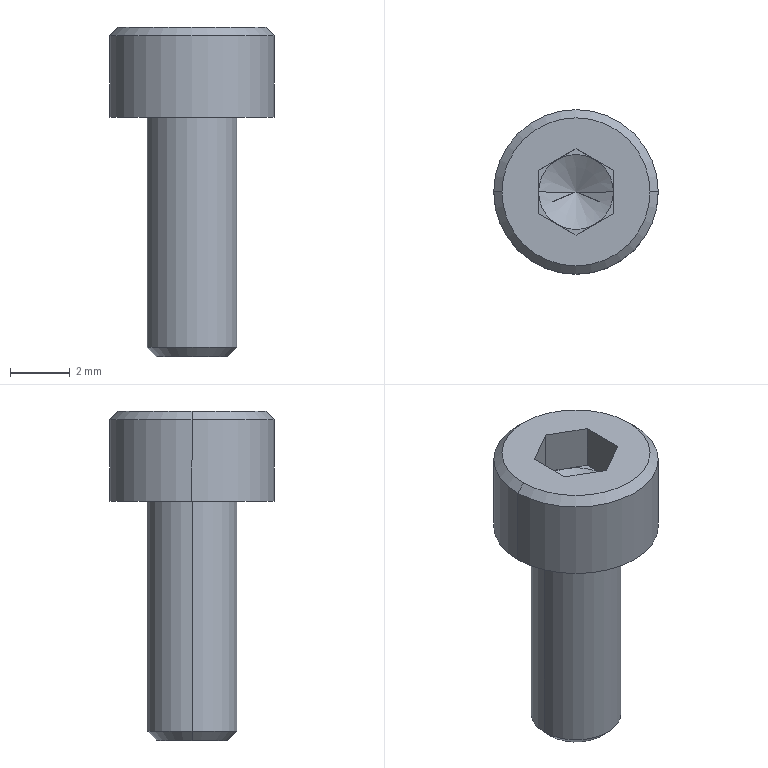Part | NX | features BREP 1 | 1 solid | 25 faces | box 5.5 x 5.5 x 11 mm | volume 117.48 mm3 | plane 15 | cone 6 | cylinder 4 | commonest cylinder face diameters 3 x2 5.5 x2
STEP:
#1=CARTESIAN_POINT('',(0.,0.,0.7783));
#2=VERTEX_POINT('',#1);
#3=CARTESIAN_POINT('',(1.25,0.,1.5));
#4=VERTEX_POINT('',#3);
#5=CARTESIAN_POINT('',(0.,0.,0.7783));
#6=DIRECTION('',(0.866,0.,0.5));
#7=VECTOR('',#6,1000.);
#8=LINE('',#5,#7);
#9=EDGE_CURVE('',#2,#4,#8,.T.);
#10=ORIENTED_EDGE('',*,*,#9,.F.);
#11=CARTESIAN_POINT('',(-1.25,0.,1.5));
#12=VERTEX_POINT('',#11);
#13=CARTESIAN_POINT('',(0.,0.,0.7783));
#14=DIRECTION('',(-0.866,0.,0.5));
#15=VECTOR('',#14,1000.);
#16=LINE('',#13,#15);
#17=EDGE_CURVE('',#2,#12,#16,.T.);
#18=ORIENTED_EDGE('',*,*,#17,.T.);
#19=CARTESIAN_POINT('',(-0.625,-1.083,1.5));
#20=VERTEX_POINT('',#19);
#21=CARTESIAN_POINT('',(0.,0.,1.5));
#22=DIRECTION('',(0.,0.,1.));
#23=DIRECTION('',(1.,0.,0.));
#24=AXIS2_PLACEMENT_3D('',#21,#22,#23);
#25=CIRCLE('',#24,1.25);
#26=EDGE_CURVE('',#12,#20,#25,.T.);
#27=ORIENTED_EDGE('',*,*,#26,.T.);
#28=CARTESIAN_POINT('',(0.625,-1.083,1.5));
#29=VERTEX_POINT('',#28);
#30=CARTESIAN_POINT('',(0.,0.,1.5));
#31=DIRECTION('',(0.,0.,1.));
#32=DIRECTION('',(1.,0.,0.));
#33=AXIS2_PLACEMENT_3D('',#30,#31,#32);
#34=CIRCLE('',#33,1.25);
#35=EDGE_CURVE('',#20,#29,#34,.T.);
#36=ORIENTED_EDGE('',*,*,#35,.T.);
#37=CARTESIAN_POINT('',(0.,0.,1.5));
#38=DIRECTION('',(0.,0.,1.));
#39=DIRECTION('',(1.,0.,0.));
#40=AXIS2_PLACEMENT_3D('',#37,#38,#39);
#41=CIRCLE('',#40,1.25);
#42=EDGE_CURVE('',#29,#4,#41,.T.);
#43=ORIENTED_EDGE('',*,*,#42,.T.);
#44=EDGE_LOOP('',(#10,#18,#27,#36,#43));
#45=FACE_BOUND('',#44,.T.);
#46=CARTESIAN_POINT('',(0.,0.,1000.778));
#47=DIRECTION('',(0.,0.,1.));
#48=DIRECTION('',(-1.,0.,0.));
#49=AXIS2_PLACEMENT_3D('',#46,#47,#48);
#50=CONICAL_SURFACE('',#49,1732.051,1.047);
#51=ADVANCED_FACE('',(#45),#50,.F.);
#52=CARTESIAN_POINT('',(2.75,0.,0.));
#53=VERTEX_POINT('',#52);
#54=CARTESIAN_POINT('',(-2.75,0.,0.));
#55=VERTEX_POINT('',#54);
#56=CARTESIAN_POINT('',(0.,0.,0.));
#57=DIRECTION('',(0.,0.,1.));
#58=DIRECTION('',(1.,0.,0.));
#59=AXIS2_PLACEMENT_3D('',#56,#57,#58);
#60=CIRCLE('',#59,2.75);
#61=EDGE_CURVE('',#53,#55,#60,.T.);
#62=ORIENTED_EDGE('',*,*,#61,.T.);
#63=CARTESIAN_POINT('',(-2.75,0.,2.725));
#64=VERTEX_POINT('',#63);
#65=CARTESIAN_POINT('',(-2.75,0.,0.));
#66=DIRECTION('',(0.,0.,1.));
#67=VECTOR('',#66,1000.);
#68=LINE('',#65,#67);
#69=EDGE_CURVE('',#55,#64,#68,.T.);
#70=ORIENTED_EDGE('',*,*,#69,.T.);
#71=CARTESIAN_POINT('',(2.75,0.,2.725));
#72=VERTEX_POINT('',#71);
#73=CARTESIAN_POINT('',(0.,0.,2.725));
#74=DIRECTION('',(0.,0.,1.));
#75=DIRECTION('',(1.,0.,0.));
#76=AXIS2_PLACEMENT_3D('',#73,#74,#75);
#77=CIRCLE('',#76,2.75);
#78=EDGE_CURVE('',#72,#64,#77,.T.);
#79=ORIENTED_EDGE('',*,*,#78,.F.);
#80=CARTESIAN_POINT('',(2.75,0.,0.));
#81=DIRECTION('',(0.,0.,1.));
#82=VECTOR('',#81,1000.);
#83=LINE('',#80,#82);
#84=EDGE_CURVE('',#53,#72,#83,.T.);
#85=ORIENTED_EDGE('',*,*,#84,.F.);
#86=EDGE_LOOP('',(#62,#70,#79,#85));
#87=FACE_BOUND('',#86,.T.);
#88=CARTESIAN_POINT('',(0.,0.,0.));
#89=DIRECTION('',(0.,0.,1.));
#90=DIRECTION('',(-1.,0.,0.));
#91=AXIS2_PLACEMENT_3D('',#88,#89,#90);
#92=CYLINDRICAL_SURFACE('',#91,2.75);
#93=ADVANCED_FACE('',(#87),#92,.T.);
#94=CARTESIAN_POINT('',(2.475,0.,3.));
#95=VERTEX_POINT('',#94);
#96=CARTESIAN_POINT('',(-2.475,0.,3.));
#97=VERTEX_POINT('',#96);
#98=CARTESIAN_POINT('',(0.,0.,3.));
#99=DIRECTION('',(0.,0.,1.));
#100=DIRECTION('',(1.,0.,0.));
#101=AXIS2_PLACEMENT_3D('',#98,#99,#100);
#102=CIRCLE('',#101,2.475);
#103=EDGE_CURVE('',#95,#97,#102,.T.);
#104=ORIENTED_EDGE('',*,*,#103,.F.);
#105=CARTESIAN_POINT('',(2.75,0.,2.725));
#106=DIRECTION('',(0.7071,0.,-0.7071));
#107=VECTOR('',#106,1000.);
#108=LINE('',#105,#107);
#109=EDGE_CURVE('',#72,#95,#108,.F.);
#110=ORIENTED_EDGE('',*,*,#109,.F.);
#111=ORIENTED_EDGE('',*,*,#78,.T.);
#112=CARTESIAN_POINT('',(-2.75,0.,2.725));
#113=DIRECTION('',(-0.7071,0.,-0.7071));
#114=VECTOR('',#113,1000.);
#115=LINE('',#112,#114);
#116=EDGE_CURVE('',#64,#97,#115,.F.);
#117=ORIENTED_EDGE('',*,*,#116,.T.);
#118=EDGE_LOOP('',(#104,#110,#111,#117));
#119=FACE_BOUND('',#118,.T.);
#120=CARTESIAN_POINT('',(0.,0.,2.725));
#121=DIRECTION('',(0.,0.,-1.));
#122=DIRECTION('',(1.,0.,0.));
#123=AXIS2_PLACEMENT_3D('',#120,#121,#122);
#124=CONICAL_SURFACE('',#123,2.75,0.7854);
#125=ADVANCED_FACE('',(#119),#124,.T.);
#126=CARTESIAN_POINT('',(1.194,0.,-8.));
#127=VERTEX_POINT('',#126);
#128=CARTESIAN_POINT('',(-1.194,0.,-8.));
#129=VERTEX_POINT('',#128);
#130=CARTESIAN_POINT('',(0.,0.,-8.));
#131=DIRECTION('',(0.,0.,1.));
#132=DIRECTION('',(1.,0.,0.));
#133=AXIS2_PLACEMENT_3D('',#130,#131,#132);
#134=CIRCLE('',#133,1.194);
#135=EDGE_CURVE('',#127,#129,#134,.T.);
#136=ORIENTED_EDGE('',*,*,#135,.T.);
#137=CARTESIAN_POINT('',(-1.5,0.,-7.694));
#138=VERTEX_POINT('',#137);
#139=CARTESIAN_POINT('',(-1.194,0.,-8.));
#140=DIRECTION('',(-0.7071,0.,0.7071));
#141=VECTOR('',#140,1000.);
#142=LINE('',#139,#141);
#143=EDGE_CURVE('',#129,#138,#142,.T.);
#144=ORIENTED_EDGE('',*,*,#143,.T.);
#145=CARTESIAN_POINT('',(1.5,0.,-7.694));
#146=VERTEX_POINT('',#145);
#147=CARTESIAN_POINT('',(0.,0.,-7.694));
#148=DIRECTION('',(0.,0.,1.));
#149=DIRECTION('',(1.,0.,0.));
#150=AXIS2_PLACEMENT_3D('',#147,#148,#149);
#151=CIRCLE('',#150,1.5);
#152=EDGE_CURVE('',#146,#138,#151,.T.);
#153=ORIENTED_EDGE('',*,*,#152,.F.);
#154=CARTESIAN_POINT('',(1.194,0.,-8.));
#155=DIRECTION('',(0.7071,0.,0.7071));
#156=VECTOR('',#155,1000.);
#157=LINE('',#154,#156);
#158=EDGE_CURVE('',#127,#146,#157,.T.);
#159=ORIENTED_EDGE('',*,*,#158,.F.);
#160=EDGE_LOOP('',(#136,#144,#153,#159));
#161=FACE_BOUND('',#160,.T.);
#162=CARTESIAN_POINT('',(0.,0.,-8.));
#163=DIRECTION('',(0.,0.,1.));
#164=DIRECTION('',(-1.,0.,0.));
#165=AXIS2_PLACEMENT_3D('',#162,#163,#164);
#166=CONICAL_SURFACE('',#165,1.194,0.7854);
#167=ADVANCED_FACE('',(#161),#166,.T.);
#168=ORIENTED_EDGE('',*,*,#152,.T.);
#169=CARTESIAN_POINT('',(-1.5,0.,0.));
#170=VERTEX_POINT('',#169);
#171=CARTESIAN_POINT('',(-1.5,0.,-8.));
#172=DIRECTION('',(0.,0.,1.));
#173=VECTOR('',#172,1000.);
#174=LINE('',#171,#173);
#175=EDGE_CURVE('',#138,#170,#174,.T.);
#176=ORIENTED_EDGE('',*,*,#175,.T.);
#177=CARTESIAN_POINT('',(1.5,0.,0.));
#178=VERTEX_POINT('',#177);
#179=CARTESIAN_POINT('',(0.,0.,0.));
#180=DIRECTION('',(0.,0.,1.));
#181=DIRECTION('',(1.,0.,0.));
#182=AXIS2_PLACEMENT_3D('',#179,#180,#181);
#183=CIRCLE('',#182,1.5);
#184=EDGE_CURVE('',#178,#170,#183,.T.);
#185=ORIENTED_EDGE('',*,*,#184,.F.);
#186=CARTESIAN_POINT('',(1.5,0.,-8.));
#187=DIRECTION('',(0.,0.,1.));
#188=VECTOR('',#187,1000.);
#189=LINE('',#186,#188);
#190=EDGE_CURVE('',#146,#178,#189,.T.);
#191=ORIENTED_EDGE('',*,*,#190,.F.);
#192=EDGE_LOOP('',(#168,#176,#185,#191));
#193=FACE_BOUND('',#192,.T.);
#194=CARTESIAN_POINT('',(0.,0.,-8.));
#195=DIRECTION('',(0.,0.,1.));
#196=DIRECTION('',(-1.,0.,0.));
#197=AXIS2_PLACEMENT_3D('',#194,#195,#196);
#198=CYLINDRICAL_SURFACE('',#197,1.5);
#199=ADVANCED_FACE('',(#193),#198,.T.);
#200=CARTESIAN_POINT('',(0.625,1.083,1.5));
#201=VERTEX_POINT('',#200);
#202=CARTESIAN_POINT('',(0.,0.,1.5));
#203=DIRECTION('',(0.,0.,1.));
#204=DIRECTION('',(1.,0.,0.));
#205=AXIS2_PLACEMENT_3D('',#202,#203,#204);
#206=CIRCLE('',#205,1.25);
#207=EDGE_CURVE('',#4,#201,#206,.T.);
#208=ORIENTED_EDGE('',*,*,#207,.F.);
#209=CARTESIAN_POINT('',(1.25,0.7217,1.5));
#210=VERTEX_POINT('',#209);
#211=CARTESIAN_POINT('',(1.25,-0.7217,1.5));
#212=DIRECTION('',(0.,1.,0.));
#213=VECTOR('',#212,1000.);
#214=LINE('',#211,#213);
#215=EDGE_CURVE('',#4,#210,#214,.T.);
#216=ORIENTED_EDGE('',*,*,#215,.T.);
#217=CARTESIAN_POINT('',(1.25,0.7217,1.5));
#218=DIRECTION('',(-0.866,0.5,0.));
#219=VECTOR('',#218,1000.);
#220=LINE('',#217,#219);
#221=EDGE_CURVE('',#210,#201,#220,.T.);
#222=ORIENTED_EDGE('',*,*,#221,.T.);
#223=EDGE_LOOP('',(#208,#216,#222));
#224=FACE_BOUND('',#223,.T.);
#225=CARTESIAN_POINT('',(0.,0.,1.5));
#226=DIRECTION('',(0.,0.,1.));
#227=DIRECTION('',(-1.,0.,0.));
#228=AXIS2_PLACEMENT_3D('',#225,#226,#227);
#229=PLANE('',#228);
#230=ADVANCED_FACE('',(#224),#229,.T.);
#231=CARTESIAN_POINT('',(-0.625,1.083,1.5));
#232=VERTEX_POINT('',#231);
#233=CARTESIAN_POINT('',(0.,0.,1.5));
#234=DIRECTION('',(0.,0.,1.));
#235=DIRECTION('',(1.,0.,0.));
#236=AXIS2_PLACEMENT_3D('',#233,#234,#235);
#237=CIRCLE('',#236,1.25);
#238=EDGE_CURVE('',#201,#232,#237,.T.);
#239=ORIENTED_EDGE('',*,*,#238,.F.);
#240=CARTESIAN_POINT('',(0.,1.443,1.5));
#241=VERTEX_POINT('',#240);
#242=CARTESIAN_POINT('',(1.25,0.7217,1.5));
#243=DIRECTION('',(-0.866,0.5,0.));
#244=VECTOR('',#243,1000.);
#245=LINE('',#242,#244);
#246=EDGE_CURVE('',#201,#241,#245,.T.);
#247=ORIENTED_EDGE('',*,*,#246,.T.);
#248=CARTESIAN_POINT('',(0.,1.443,1.5));
#249=DIRECTION('',(-0.866,-0.5,0.));
#250=VECTOR('',#249,1000.);
#251=LINE('',#248,#250);
#252=EDGE_CURVE('',#241,#232,#251,.T.);
#253=ORIENTED_EDGE('',*,*,#252,.T.);
#254=EDGE_LOOP('',(#239,#247,#253));
#255=FACE_BOUND('',#254,.T.);
#256=CARTESIAN_POINT('',(0.,0.,1.5));
#257=DIRECTION('',(0.,0.,1.));
#258=DIRECTION('',(-1.,0.,0.));
#259=AXIS2_PLACEMENT_3D('',#256,#257,#258);
#260=PLANE('',#259);
#261=ADVANCED_FACE('',(#255),#260,.T.);
#262=CARTESIAN_POINT('',(0.,0.,1.5));
#263=DIRECTION('',(0.,0.,1.));
#264=DIRECTION('',(1.,0.,0.));
#265=AXIS2_PLACEMENT_3D('',#262,#263,#264);
#266=CIRCLE('',#265,1.25);
#267=EDGE_CURVE('',#232,#12,#266,.T.);
#268=ORIENTED_EDGE('',*,*,#267,.F.);
#269=CARTESIAN_POINT('',(-1.25,0.7217,1.5));
#270=VERTEX_POINT('',#269);
#271=CARTESIAN_POINT('',(0.,1.443,1.5));
#272=DIRECTION('',(-0.866,-0.5,0.));
#273=VECTOR('',#272,1000.);
#274=LINE('',#271,#273);
#275=EDGE_CURVE('',#232,#270,#274,.T.);
#276=ORIENTED_EDGE('',*,*,#275,.T.);
#277=CARTESIAN_POINT('',(-1.25,0.7217,1.5));
#278=DIRECTION('',(0.,-1.,0.));
#279=VECTOR('',#278,1000.);
#280=LINE('',#277,#279);
#281=EDGE_CURVE('',#270,#12,#280,.T.);
#282=ORIENTED_EDGE('',*,*,#281,.T.);
#283=EDGE_LOOP('',(#268,#276,#282));
#284=FACE_BOUND('',#283,.T.);
#285=CARTESIAN_POINT('',(0.,0.,1.5));
#286=DIRECTION('',(0.,0.,1.));
#287=DIRECTION('',(-1.,0.,0.));
#288=AXIS2_PLACEMENT_3D('',#285,#286,#287);
#289=PLANE('',#288);
#290=ADVANCED_FACE('',(#284),#289,.T.);
#291=ORIENTED_EDGE('',*,*,#26,.F.);
#292=CARTESIAN_POINT('',(-1.25,-0.7217,1.5));
#293=VERTEX_POINT('',#292);
#294=CARTESIAN_POINT('',(-1.25,0.7217,1.5));
#295=DIRECTION('',(0.,-1.,0.));
#296=VECTOR('',#295,1000.);
#297=LINE('',#294,#296);
#298=EDGE_CURVE('',#12,#293,#297,.T.);
#299=ORIENTED_EDGE('',*,*,#298,.T.);
#300=CARTESIAN_POINT('',(-1.25,-0.7217,1.5));
#301=DIRECTION('',(0.866,-0.5,0.));
#302=VECTOR('',#301,1000.);
#303=LINE('',#300,#302);
#304=EDGE_CURVE('',#293,#20,#303,.T.);
#305=ORIENTED_EDGE('',*,*,#304,.T.);
#306=EDGE_LOOP('',(#291,#299,#305));
#307=FACE_BOUND('',#306,.T.);
#308=CARTESIAN_POINT('',(0.,0.,1.5));
#309=DIRECTION('',(0.,0.,1.));
#310=DIRECTION('',(-1.,0.,0.));
#311=AXIS2_PLACEMENT_3D('',#308,#309,#310);
#312=PLANE('',#311);
#313=ADVANCED_FACE('',(#307),#312,.T.);
#314=ORIENTED_EDGE('',*,*,#35,.F.);
#315=CARTESIAN_POINT('',(0.,-1.443,1.5));
#316=VERTEX_POINT('',#315);
#317=CARTESIAN_POINT('',(-1.25,-0.7217,1.5));
#318=DIRECTION('',(0.866,-0.5,0.));
#319=VECTOR('',#318,1000.);
#320=LINE('',#317,#319);
#321=EDGE_CURVE('',#20,#316,#320,.T.);
#322=ORIENTED_EDGE('',*,*,#321,.T.);
#323=CARTESIAN_POINT('',(0.,-1.443,1.5));
#324=DIRECTION('',(0.866,0.5,0.));
#325=VECTOR('',#324,1000.);
#326=LINE('',#323,#325);
#327=EDGE_CURVE('',#316,#29,#326,.T.);
#328=ORIENTED_EDGE('',*,*,#327,.T.);
#329=EDGE_LOOP('',(#314,#322,#328));
#330=FACE_BOUND('',#329,.T.);
#331=CARTESIAN_POINT('',(0.,0.,1.5));
#332=DIRECTION('',(0.,0.,1.));
#333=DIRECTION('',(-1.,0.,0.));
#334=AXIS2_PLACEMENT_3D('',#331,#332,#333);
#335=PLANE('',#334);
#336=ADVANCED_FACE('',(#330),#335,.T.);
#337=ORIENTED_EDGE('',*,*,#175,.F.);
#338=CARTESIAN_POINT('',(0.,0.,-7.694));
#339=DIRECTION('',(0.,0.,1.));
#340=DIRECTION('',(1.,0.,0.));
#341=AXIS2_PLACEMENT_3D('',#338,#339,#340);
#342=CIRCLE('',#341,1.5);
#343=EDGE_CURVE('',#138,#146,#342,.T.);
#344=ORIENTED_EDGE('',*,*,#343,.T.);
#345=ORIENTED_EDGE('',*,*,#190,.T.);
#346=CARTESIAN_POINT('',(0.,0.,0.));
#347=DIRECTION('',(0.,0.,1.));
#348=DIRECTION('',(1.,0.,0.));
#349=AXIS2_PLACEMENT_3D('',#346,#347,#348);
#350=CIRCLE('',#349,1.5);
#351=EDGE_CURVE('',#170,#178,#350,.T.);
#352=ORIENTED_EDGE('',*,*,#351,.F.);
#353=EDGE_LOOP('',(#337,#344,#345,#352));
#354=FACE_BOUND('',#353,.T.);
#355=CARTESIAN_POINT('',(0.,0.,-8.));
#356=DIRECTION('',(0.,0.,1.));
#357=DIRECTION('',(-1.,0.,0.));
#358=AXIS2_PLACEMENT_3D('',#355,#356,#357);
#359=CYLINDRICAL_SURFACE('',#358,1.5);
#360=ADVANCED_FACE('',(#354),#359,.T.);
#361=ORIENTED_EDGE('',*,*,#143,.F.);
#362=CARTESIAN_POINT('',(0.,0.,-8.));
#363=DIRECTION('',(0.,0.,1.));
#364=DIRECTION('',(1.,0.,0.));
#365=AXIS2_PLACEMENT_3D('',#362,#363,#364);
#366=CIRCLE('',#365,1.194);
#367=EDGE_CURVE('',#129,#127,#366,.T.);
#368=ORIENTED_EDGE('',*,*,#367,.T.);
#369=ORIENTED_EDGE('',*,*,#158,.T.);
#370=ORIENTED_EDGE('',*,*,#343,.F.);
#371=EDGE_LOOP('',(#361,#368,#369,#370));
#372=FACE_BOUND('',#371,.T.);
#373=CARTESIAN_POINT('',(0.,0.,-8.));
#374=DIRECTION('',(0.,0.,1.));
#375=DIRECTION('',(-1.,0.,0.));
#376=AXIS2_PLACEMENT_3D('',#373,#374,#375);
#377=CONICAL_SURFACE('',#376,1.194,0.7854);
#378=ADVANCED_FACE('',(#372),#377,.T.);
#379=ORIENTED_EDGE('',*,*,#135,.F.);
#380=ORIENTED_EDGE('',*,*,#367,.F.);
#381=EDGE_LOOP('',(#379,#380));
#382=FACE_BOUND('',#381,.T.);
#383=CARTESIAN_POINT('',(0.,1.194,-8.));
#384=DIRECTION('',(0.,0.,1.));
#385=DIRECTION('',(-1.,0.,0.));
#386=AXIS2_PLACEMENT_3D('',#383,#384,#385);
#387=PLANE('',#386);
#388=ADVANCED_FACE('',(#382),#387,.F.);
#389=CARTESIAN_POINT('',(0.,-1.443,3.));
#390=VERTEX_POINT('',#389);
#391=CARTESIAN_POINT('',(1.25,-0.7217,3.));
#392=VERTEX_POINT('',#391);
#393=CARTESIAN_POINT('',(0.,-1.443,3.));
#394=DIRECTION('',(0.866,0.5,0.));
#395=VECTOR('',#394,1000.);
#396=LINE('',#393,#395);
#397=EDGE_CURVE('',#390,#392,#396,.T.);
#398=ORIENTED_EDGE('',*,*,#397,.F.);
#399=CARTESIAN_POINT('',(-1.25,-0.7217,3.));
#400=VERTEX_POINT('',#399);
#401=CARTESIAN_POINT('',(-1.25,-0.7217,3.));
#402=DIRECTION('',(0.866,-0.5,0.));
#403=VECTOR('',#402,1000.);
#404=LINE('',#401,#403);
#405=EDGE_CURVE('',#400,#390,#404,.T.);
#406=ORIENTED_EDGE('',*,*,#405,.F.);
#407=CARTESIAN_POINT('',(-1.25,0.7217,3.));
#408=VERTEX_POINT('',#407);
#409=CARTESIAN_POINT('',(-1.25,0.7217,3.));
#410=DIRECTION('',(0.,-1.,0.));
#411=VECTOR('',#410,1000.);
#412=LINE('',#409,#411);
#413=EDGE_CURVE('',#408,#400,#412,.T.);
#414=ORIENTED_EDGE('',*,*,#413,.F.);
#415=CARTESIAN_POINT('',(0.,1.443,3.));
#416=VERTEX_POINT('',#415);
#417=CARTESIAN_POINT('',(0.,1.443,3.));
#418=DIRECTION('',(-0.866,-0.5,0.));
#419=VECTOR('',#418,1000.);
#420=LINE('',#417,#419);
#421=EDGE_CURVE('',#416,#408,#420,.T.);
#422=ORIENTED_EDGE('',*,*,#421,.F.);
#423=CARTESIAN_POINT('',(1.25,0.7217,3.));
#424=VERTEX_POINT('',#423);
#425=CARTESIAN_POINT('',(1.25,0.7217,3.));
#426=DIRECTION('',(-0.866,0.5,0.));
#427=VECTOR('',#426,1000.);
#428=LINE('',#425,#427);
#429=EDGE_CURVE('',#424,#416,#428,.T.);
#430=ORIENTED_EDGE('',*,*,#429,.F.);
#431=CARTESIAN_POINT('',(1.25,-0.7217,3.));
#432=DIRECTION('',(0.,1.,0.));
#433=VECTOR('',#432,1000.);
#434=LINE('',#431,#433);
#435=EDGE_CURVE('',#392,#424,#434,.T.);
#436=ORIENTED_EDGE('',*,*,#435,.F.);
#437=EDGE_LOOP('',(#398,#406,#414,#422,#430,#436));
#438=FACE_BOUND('',#437,.T.);
#439=CARTESIAN_POINT('',(0.,0.,3.));
#440=DIRECTION('',(0.,0.,1.));
#441=DIRECTION('',(1.,0.,0.));
#442=AXIS2_PLACEMENT_3D('',#439,#440,#441);
#443=CIRCLE('',#442,2.475);
#444=EDGE_CURVE('',#97,#95,#443,.T.);
#445=ORIENTED_EDGE('',*,*,#444,.T.);
#446=ORIENTED_EDGE('',*,*,#103,.T.);
#447=EDGE_LOOP('',(#445,#446));
#448=FACE_BOUND('',#447,.T.);
#449=CARTESIAN_POINT('',(0.,0.,3.));
#450=DIRECTION('',(0.,0.,-1.));
#451=DIRECTION('',(1.,0.,0.));
#452=AXIS2_PLACEMENT_3D('',#449,#450,#451);
#453=PLANE('',#452);
#454=ADVANCED_FACE('',(#438,#448),#453,.F.);
#455=ORIENTED_EDGE('',*,*,#109,.T.);
#456=ORIENTED_EDGE('',*,*,#444,.F.);
#457=ORIENTED_EDGE('',*,*,#116,.F.);
#458=CARTESIAN_POINT('',(0.,0.,2.725));
#459=DIRECTION('',(0.,0.,1.));
#460=DIRECTION('',(1.,0.,0.));
#461=AXIS2_PLACEMENT_3D('',#458,#459,#460);
#462=CIRCLE('',#461,2.75);
#463=EDGE_CURVE('',#64,#72,#462,.T.);
#464=ORIENTED_EDGE('',*,*,#463,.T.);
#465=EDGE_LOOP('',(#455,#456,#457,#464));
#466=FACE_BOUND('',#465,.T.);
#467=CARTESIAN_POINT('',(0.,0.,2.725));
#468=DIRECTION('',(0.,0.,-1.));
#469=DIRECTION('',(1.,0.,0.));
#470=AXIS2_PLACEMENT_3D('',#467,#468,#469);
#471=CONICAL_SURFACE('',#470,2.75,0.7854);
#472=ADVANCED_FACE('',(#466),#471,.T.);
#473=ORIENTED_EDGE('',*,*,#69,.F.);
#474=CARTESIAN_POINT('',(0.,0.,0.));
#475=DIRECTION('',(0.,0.,1.));
#476=DIRECTION('',(1.,0.,0.));
#477=AXIS2_PLACEMENT_3D('',#474,#475,#476);
#478=CIRCLE('',#477,2.75);
#479=EDGE_CURVE('',#55,#53,#478,.T.);
#480=ORIENTED_EDGE('',*,*,#479,.T.);
#481=ORIENTED_EDGE('',*,*,#84,.T.);
#482=ORIENTED_EDGE('',*,*,#463,.F.);
#483=EDGE_LOOP('',(#473,#480,#481,#482));
#484=FACE_BOUND('',#483,.T.);
#485=CARTESIAN_POINT('',(0.,0.,0.));
#486=DIRECTION('',(0.,0.,1.));
#487=DIRECTION('',(-1.,0.,0.));
#488=AXIS2_PLACEMENT_3D('',#485,#486,#487);
#489=CYLINDRICAL_SURFACE('',#488,2.75);
#490=ADVANCED_FACE('',(#484),#489,.T.);
#491=ORIENTED_EDGE('',*,*,#184,.T.);
#492=ORIENTED_EDGE('',*,*,#351,.T.);
#493=EDGE_LOOP('',(#491,#492));
#494=FACE_BOUND('',#493,.T.);
#495=ORIENTED_EDGE('',*,*,#61,.F.);
#496=ORIENTED_EDGE('',*,*,#479,.F.);
#497=EDGE_LOOP('',(#495,#496));
#498=FACE_BOUND('',#497,.T.);
#499=CARTESIAN_POINT('',(0.,2.75,0.));
#500=DIRECTION('',(0.,0.,1.));
#501=DIRECTION('',(-1.,0.,0.));
#502=AXIS2_PLACEMENT_3D('',#499,#500,#501);
#503=PLANE('',#502);
#504=ADVANCED_FACE('',(#494,#498),#503,.F.);
#505=ORIENTED_EDGE('',*,*,#405,.T.);
#506=CARTESIAN_POINT('',(0.,-1.443,1.5));
#507=DIRECTION('',(0.,0.,1.));
#508=VECTOR('',#507,1000.);
#509=LINE('',#506,#508);
#510=EDGE_CURVE('',#316,#390,#509,.T.);
#511=ORIENTED_EDGE('',*,*,#510,.F.);
#512=ORIENTED_EDGE('',*,*,#321,.F.);
#513=ORIENTED_EDGE('',*,*,#304,.F.);
#514=CARTESIAN_POINT('',(-1.25,-0.7217,1.5));
#515=DIRECTION('',(0.,0.,1.));
#516=VECTOR('',#515,1000.);
#517=LINE('',#514,#516);
#518=EDGE_CURVE('',#293,#400,#517,.T.);
#519=ORIENTED_EDGE('',*,*,#518,.T.);
#520=EDGE_LOOP('',(#505,#511,#512,#513,#519));
#521=FACE_BOUND('',#520,.T.);
#522=CARTESIAN_POINT('',(-1.25,-0.7217,1.5));
#523=DIRECTION('',(-0.5,-0.866,0.));
#524=DIRECTION('',(-0.866,0.5,0.));
#525=AXIS2_PLACEMENT_3D('',#522,#523,#524);
#526=PLANE('',#525);
#527=ADVANCED_FACE('',(#521),#526,.F.);
#528=ORIENTED_EDGE('',*,*,#413,.T.);
#529=ORIENTED_EDGE('',*,*,#518,.F.);
#530=ORIENTED_EDGE('',*,*,#298,.F.);
#531=ORIENTED_EDGE('',*,*,#281,.F.);
#532=CARTESIAN_POINT('',(-1.25,0.7217,1.5));
#533=DIRECTION('',(0.,0.,1.));
#534=VECTOR('',#533,1000.);
#535=LINE('',#532,#534);
#536=EDGE_CURVE('',#270,#408,#535,.T.);
#537=ORIENTED_EDGE('',*,*,#536,.T.);
#538=EDGE_LOOP('',(#528,#529,#530,#531,#537));
#539=FACE_BOUND('',#538,.T.);
#540=CARTESIAN_POINT('',(-1.25,0.7217,1.5));
#541=DIRECTION('',(-1.,0.,0.));
#542=DIRECTION('',(0.,0.,-1.));
#543=AXIS2_PLACEMENT_3D('',#540,#541,#542);
#544=PLANE('',#543);
#545=ADVANCED_FACE('',(#539),#544,.F.);
#546=ORIENTED_EDGE('',*,*,#421,.T.);
#547=ORIENTED_EDGE('',*,*,#536,.F.);
#548=ORIENTED_EDGE('',*,*,#275,.F.);
#549=ORIENTED_EDGE('',*,*,#252,.F.);
#550=CARTESIAN_POINT('',(0.,1.443,1.5));
#551=DIRECTION('',(0.,0.,1.));
#552=VECTOR('',#551,1000.);
#553=LINE('',#550,#552);
#554=EDGE_CURVE('',#241,#416,#553,.T.);
#555=ORIENTED_EDGE('',*,*,#554,.T.);
#556=EDGE_LOOP('',(#546,#547,#548,#549,#555));
#557=FACE_BOUND('',#556,.T.);
#558=CARTESIAN_POINT('',(0.,1.443,1.5));
#559=DIRECTION('',(-0.5,0.866,0.));
#560=DIRECTION('',(0.866,0.5,0.));
#561=AXIS2_PLACEMENT_3D('',#558,#559,#560);
#562=PLANE('',#561);
#563=ADVANCED_FACE('',(#557),#562,.F.);
#564=ORIENTED_EDGE('',*,*,#429,.T.);
#565=ORIENTED_EDGE('',*,*,#554,.F.);
#566=ORIENTED_EDGE('',*,*,#246,.F.);
#567=ORIENTED_EDGE('',*,*,#221,.F.);
#568=CARTESIAN_POINT('',(1.25,0.7217,1.5));
#569=DIRECTION('',(0.,0.,1.));
#570=VECTOR('',#569,1000.);
#571=LINE('',#568,#570);
#572=EDGE_CURVE('',#210,#424,#571,.T.);
#573=ORIENTED_EDGE('',*,*,#572,.T.);
#574=EDGE_LOOP('',(#564,#565,#566,#567,#573));
#575=FACE_BOUND('',#574,.T.);
#576=CARTESIAN_POINT('',(1.25,0.7217,1.5));
#577=DIRECTION('',(0.5,0.866,0.));
#578=DIRECTION('',(0.866,-0.5,0.));
#579=AXIS2_PLACEMENT_3D('',#576,#577,#578);
#580=PLANE('',#579);
#581=ADVANCED_FACE('',(#575),#580,.F.);
#582=ORIENTED_EDGE('',*,*,#435,.T.);
#583=ORIENTED_EDGE('',*,*,#572,.F.);
#584=ORIENTED_EDGE('',*,*,#215,.F.);
#585=CARTESIAN_POINT('',(1.25,-0.7217,1.5));
#586=VERTEX_POINT('',#585);
#587=CARTESIAN_POINT('',(1.25,-0.7217,1.5));
#588=DIRECTION('',(0.,1.,0.));
#589=VECTOR('',#588,1000.);
#590=LINE('',#587,#589);
#591=EDGE_CURVE('',#586,#4,#590,.T.);
#592=ORIENTED_EDGE('',*,*,#591,.F.);
#593=CARTESIAN_POINT('',(1.25,-0.7217,1.5));
#594=DIRECTION('',(0.,0.,1.));
#595=VECTOR('',#594,1000.);
#596=LINE('',#593,#595);
#597=EDGE_CURVE('',#586,#392,#596,.T.);
#598=ORIENTED_EDGE('',*,*,#597,.T.);
#599=EDGE_LOOP('',(#582,#583,#584,#592,#598));
#600=FACE_BOUND('',#599,.T.);
#601=CARTESIAN_POINT('',(1.25,-0.7217,1.5));
#602=DIRECTION('',(1.,0.,0.));
#603=DIRECTION('',(0.,0.,1.));
#604=AXIS2_PLACEMENT_3D('',#601,#602,#603);
#605=PLANE('',#604);
#606=ADVANCED_FACE('',(#600),#605,.F.);
#607=ORIENTED_EDGE('',*,*,#397,.T.);
#608=ORIENTED_EDGE('',*,*,#597,.F.);
#609=CARTESIAN_POINT('',(0.,-1.443,1.5));
#610=DIRECTION('',(0.866,0.5,0.));
#611=VECTOR('',#610,1000.);
#612=LINE('',#609,#611);
#613=EDGE_CURVE('',#29,#586,#612,.T.);
#614=ORIENTED_EDGE('',*,*,#613,.F.);
#615=ORIENTED_EDGE('',*,*,#327,.F.);
#616=ORIENTED_EDGE('',*,*,#510,.T.);
#617=EDGE_LOOP('',(#607,#608,#614,#615,#616));
#618=FACE_BOUND('',#617,.T.);
#619=CARTESIAN_POINT('',(0.,-1.443,1.5));
#620=DIRECTION('',(0.5,-0.866,0.));
#621=DIRECTION('',(-0.866,-0.5,0.));
#622=AXIS2_PLACEMENT_3D('',#619,#620,#621);
#623=PLANE('',#622);
#624=ADVANCED_FACE('',(#618),#623,.F.);
#625=ORIENTED_EDGE('',*,*,#42,.F.);
#626=ORIENTED_EDGE('',*,*,#613,.T.);
#627=ORIENTED_EDGE('',*,*,#591,.T.);
#628=EDGE_LOOP('',(#625,#626,#627));
#629=FACE_BOUND('',#628,.T.);
#630=CARTESIAN_POINT('',(0.,0.,1.5));
#631=DIRECTION('',(0.,0.,1.));
#632=DIRECTION('',(-1.,0.,0.));
#633=AXIS2_PLACEMENT_3D('',#630,#631,#632);
#634=PLANE('',#633);
#635=ADVANCED_FACE('',(#629),#634,.T.);
#636=ORIENTED_EDGE('',*,*,#17,.F.);
#637=ORIENTED_EDGE('',*,*,#9,.T.);
#638=ORIENTED_EDGE('',*,*,#207,.T.);
#639=ORIENTED_EDGE('',*,*,#238,.T.);
#640=ORIENTED_EDGE('',*,*,#267,.T.);
#641=EDGE_LOOP('',(#636,#637,#638,#639,#640));
#642=FACE_BOUND('',#641,.T.);
#643=CARTESIAN_POINT('',(0.,0.,1000.778));
#644=DIRECTION('',(0.,0.,1.));
#645=DIRECTION('',(-1.,0.,0.));
#646=AXIS2_PLACEMENT_3D('',#643,#644,#645);
#647=CONICAL_SURFACE('',#646,1732.051,1.047);
#648=ADVANCED_FACE('',(#642),#647,.F.);
#649=CLOSED_SHELL('',(#51,#93,#125,#167,#199,#230,#261,#290,#313,#336,#360,#378,#388,#454,#472,#490,#504,#527,#545,#563,#581,#606,#624,#635,#648));
#650=MANIFOLD_SOLID_BREP('',#649);
#651=(LENGTH_UNIT()NAMED_UNIT(*)SI_UNIT(.MILLI.,.METRE.));
#652=UNCERTAINTY_MEASURE_WITH_UNIT(LENGTH_MEASURE(0.00001),#651,'','');
#653=(NAMED_UNIT(*)PLANE_ANGLE_UNIT()SI_UNIT($,.RADIAN.));
#654=(NAMED_UNIT(*)SI_UNIT($,.STERADIAN.)SOLID_ANGLE_UNIT());
#655=(GEOMETRIC_REPRESENTATION_CONTEXT(3)GLOBAL_UNCERTAINTY_ASSIGNED_CONTEXT((#652))GLOBAL_UNIT_ASSIGNED_CONTEXT((#651,#653,#654))REPRESENTATION_CONTEXT('',''));
#656=ADVANCED_BREP_SHAPE_REPRESENTATION('',(#650),#655);